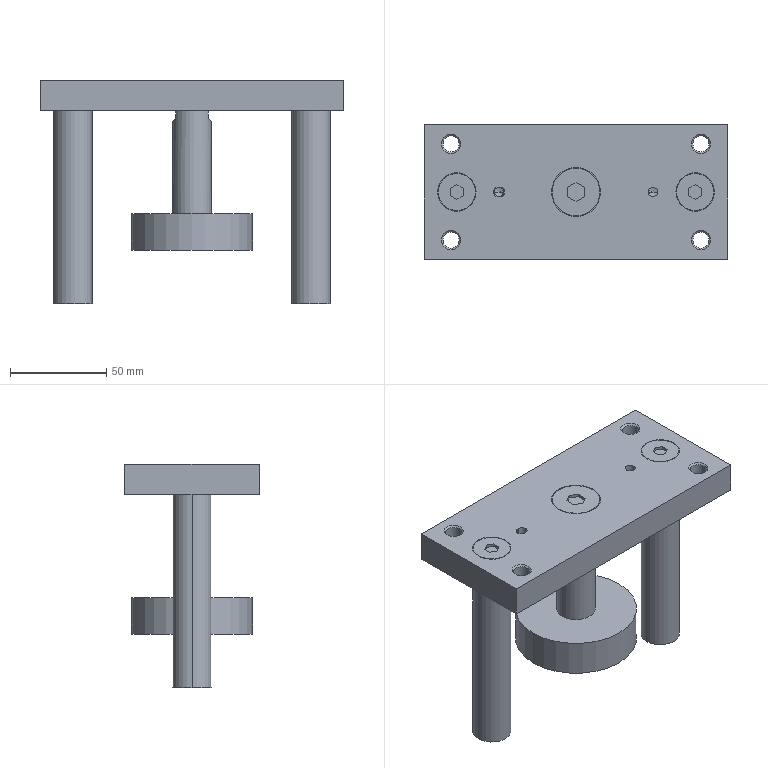Part | 1 solid | 100 faces | box 158 x 70 x 116.5 mm | volume 311829 mm3 | plane 45 | cylinder 35 | cone 20 | commonest cylinder face diameters 20 x10 8.376 x8 5 x7 19.4 x4 24.9 x2 25.5 x2